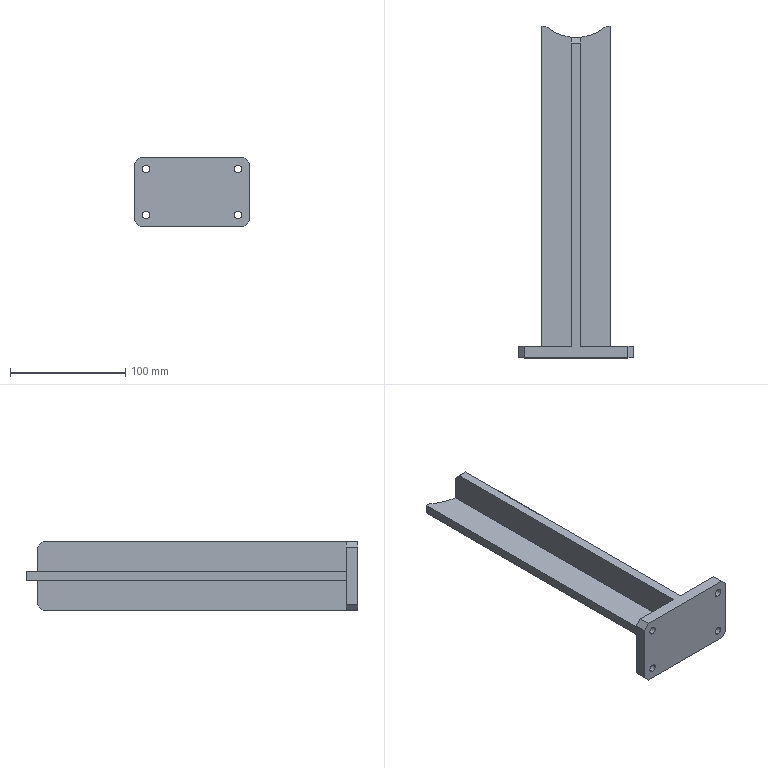Part | STEP file | Tube support base-extension | 1 solid | 36 faces | box 100 x 288 x 60 mm | volume 299980 mm3 | plane 23 | cylinder 11 | cone 2 | commonest cylinder face diameters 6.6 x8 10 x2 80 x1